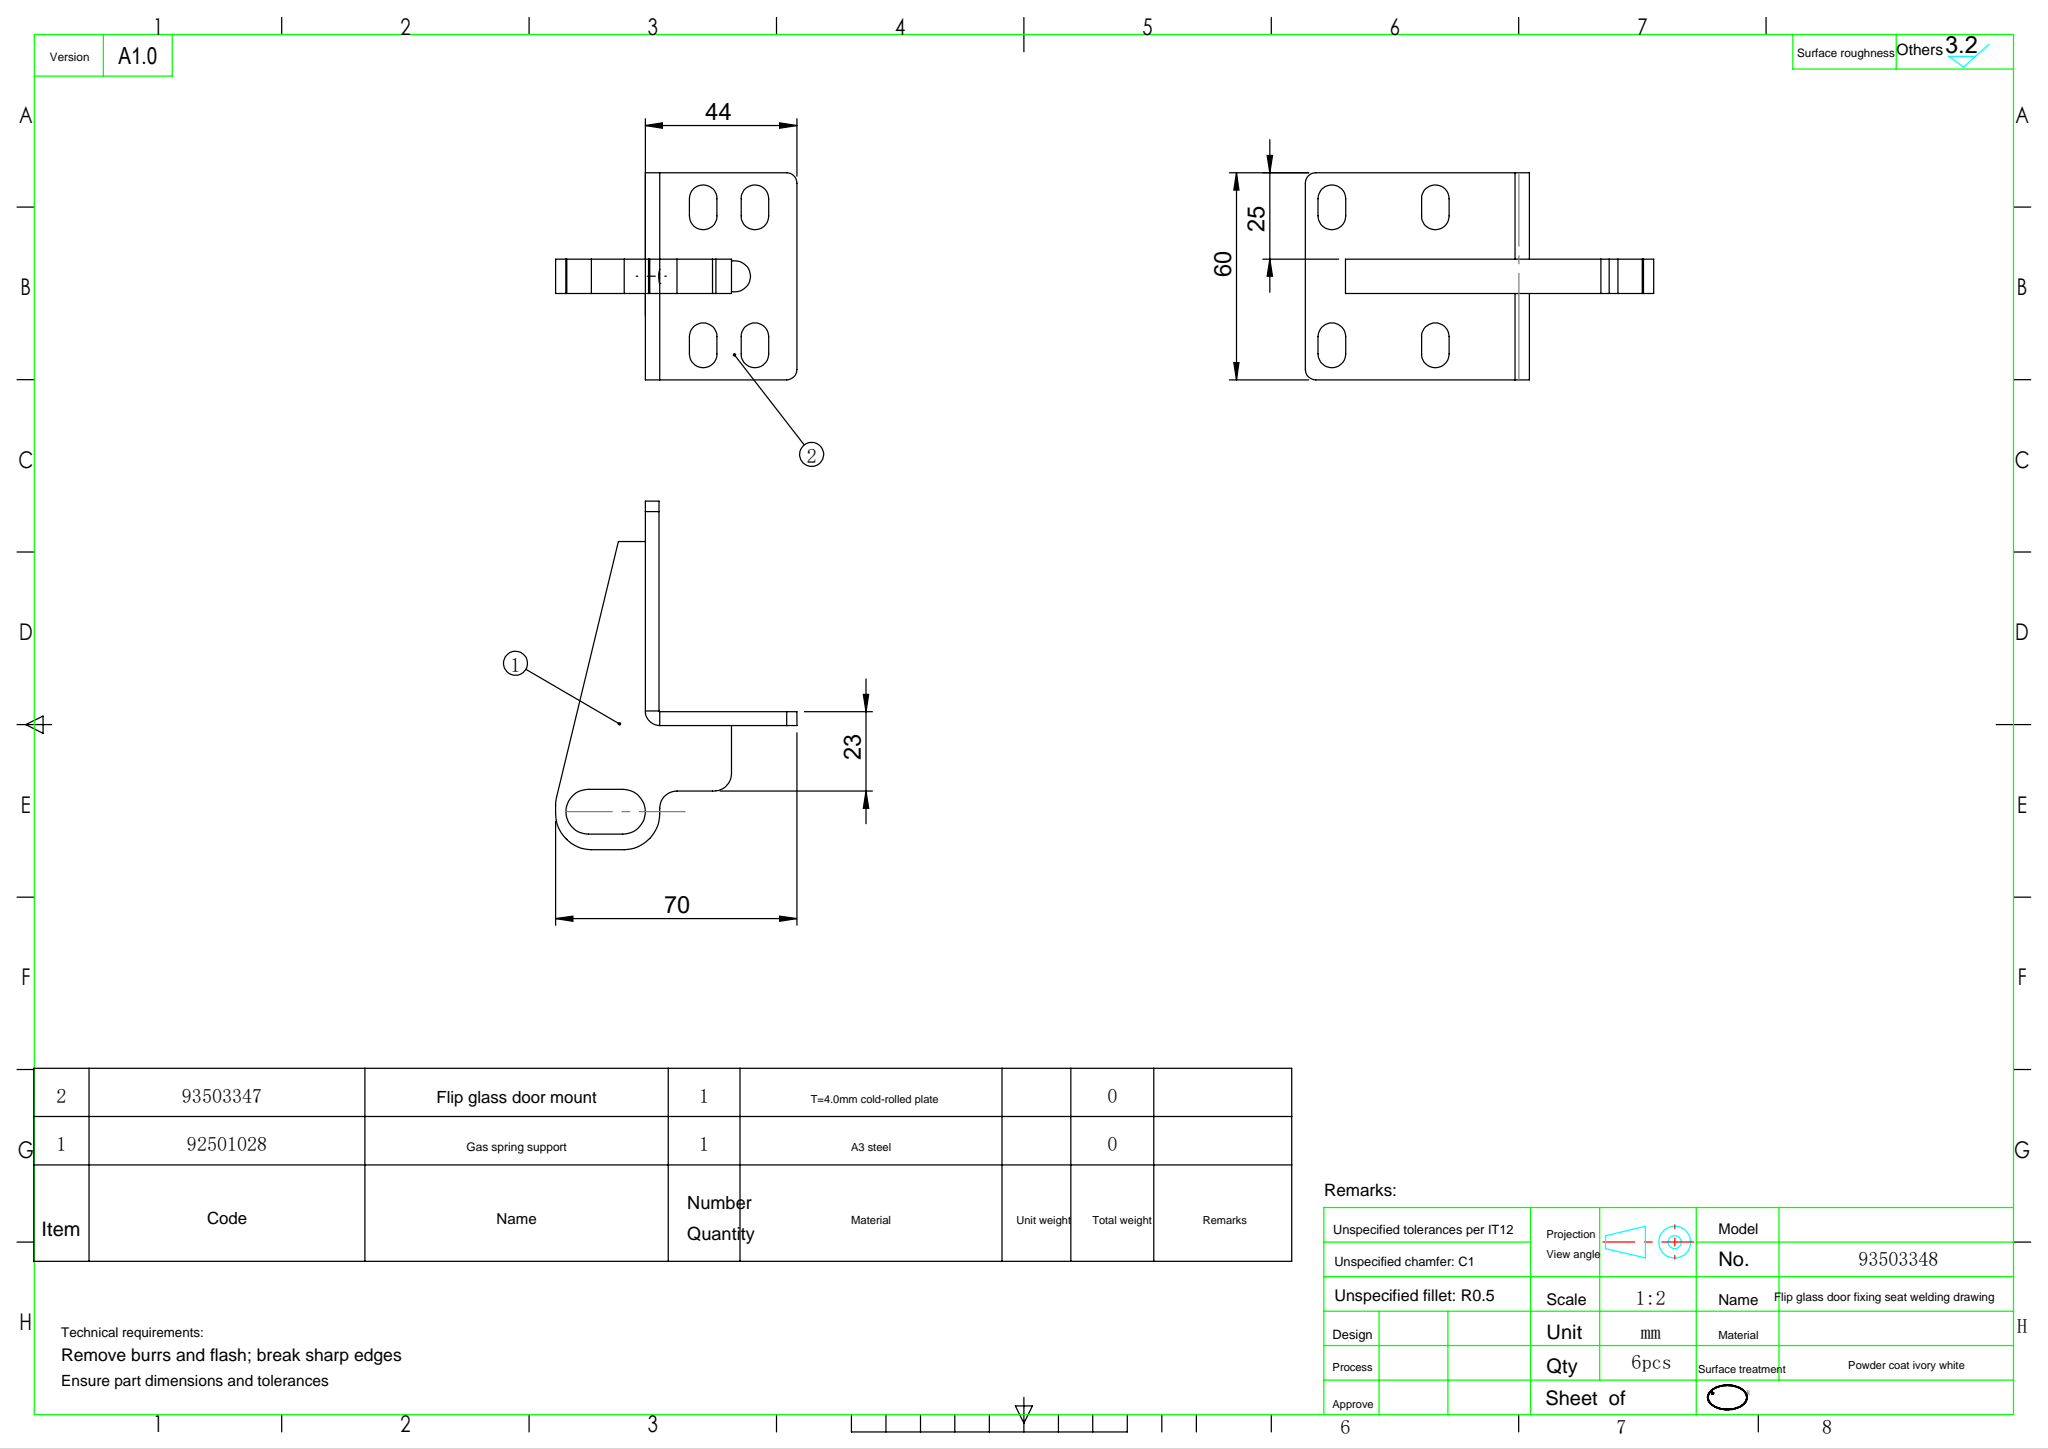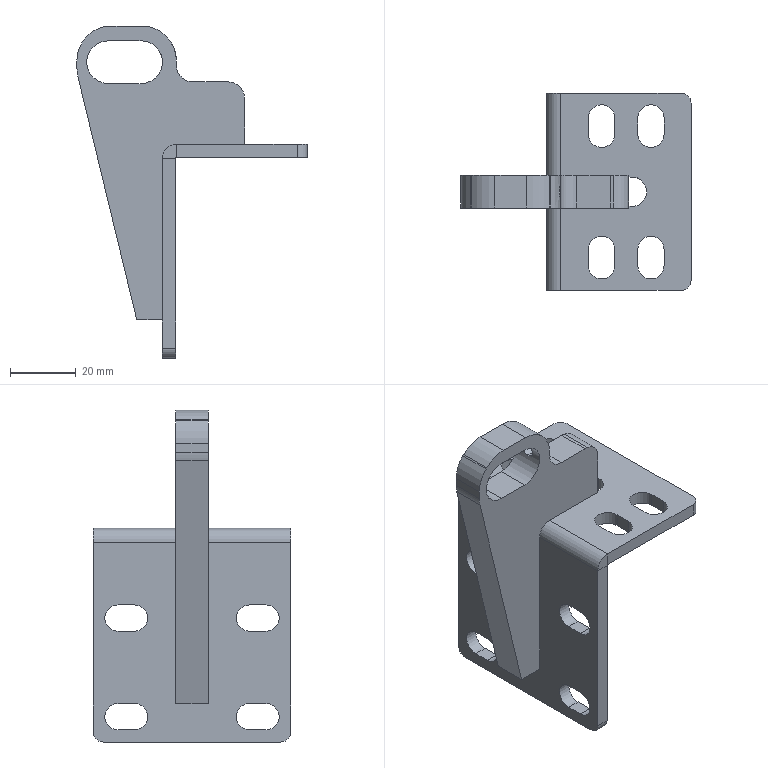Part | SolidWorks | 2 solids | 88 faces | box 70 x 60 x 101 mm | volume 39766 mm3 | plane 45 | cylinder 43 | commonest cylinder face diameters 8 x16 9 x8 20 x6 6 x4 4.2 x2 8.4 x2